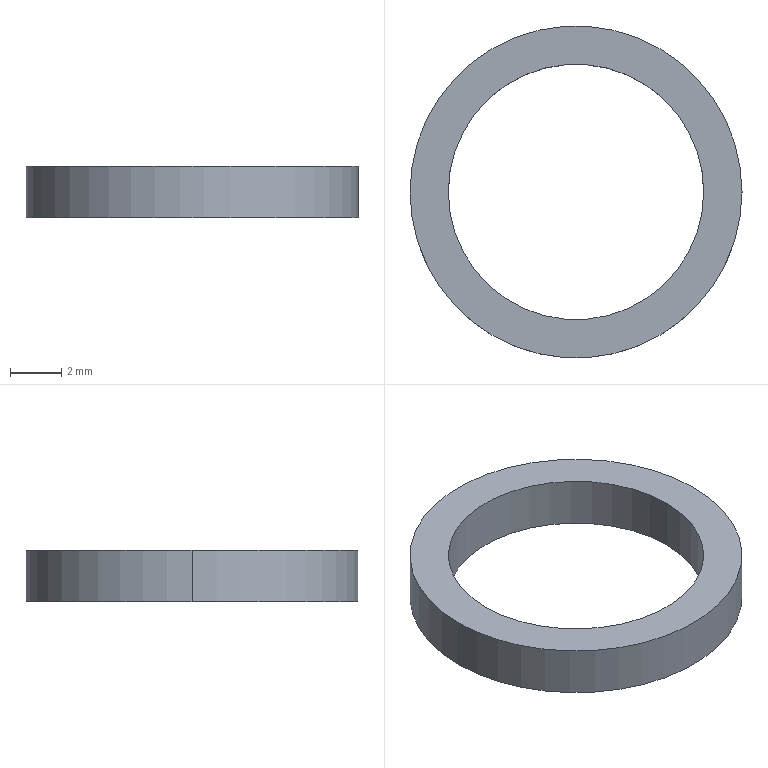Part | STEP file | 11-FG-B04311 | 1 solid | 6 faces | box 13 x 13 x 2 mm | volume 108.385 mm3 | cylinder 4 | plane 2 | commonest cylinder face diameters 10 x2 13 x2
STEP:
#1=CARTESIAN_POINT('',(-5.,0.,2.));
#2=VERTEX_POINT('',#1);
#3=CARTESIAN_POINT('',(5.,0.,2.));
#4=VERTEX_POINT('',#3);
#5=CARTESIAN_POINT('',(0.,0.,2.));
#6=DIRECTION('',(0.,0.,1.));
#7=DIRECTION('',(1.,0.,0.));
#8=AXIS2_PLACEMENT_3D('',#5,#6,#7);
#9=CIRCLE('',#8,5.);
#10=EDGE_CURVE('',#2,#4,#9,.T.);
#11=ORIENTED_EDGE('',*,*,#10,.T.);
#12=CARTESIAN_POINT('',(5.,0.,0.));
#13=VERTEX_POINT('',#12);
#14=CARTESIAN_POINT('',(5.,0.,2.));
#15=DIRECTION('',(0.,0.,-1.));
#16=VECTOR('',#15,1000.);
#17=LINE('',#14,#16);
#18=EDGE_CURVE('',#4,#13,#17,.T.);
#19=ORIENTED_EDGE('',*,*,#18,.T.);
#20=CARTESIAN_POINT('',(-5.,0.,0.));
#21=VERTEX_POINT('',#20);
#22=CARTESIAN_POINT('',(0.,0.,0.));
#23=DIRECTION('',(0.,0.,1.));
#24=DIRECTION('',(1.,0.,0.));
#25=AXIS2_PLACEMENT_3D('',#22,#23,#24);
#26=CIRCLE('',#25,5.);
#27=EDGE_CURVE('',#21,#13,#26,.T.);
#28=ORIENTED_EDGE('',*,*,#27,.F.);
#29=CARTESIAN_POINT('',(-5.,0.,2.));
#30=DIRECTION('',(0.,0.,-1.));
#31=VECTOR('',#30,1000.);
#32=LINE('',#29,#31);
#33=EDGE_CURVE('',#2,#21,#32,.T.);
#34=ORIENTED_EDGE('',*,*,#33,.F.);
#35=EDGE_LOOP('',(#11,#19,#28,#34));
#36=FACE_OUTER_BOUND('',#35,.T.);
#37=CARTESIAN_POINT('',(0.,0.,2.));
#38=DIRECTION('',(0.,0.,-1.));
#39=DIRECTION('',(-1.,0.,0.));
#40=AXIS2_PLACEMENT_3D('',#37,#38,#39);
#41=CYLINDRICAL_SURFACE('',#40,5.);
#42=ADVANCED_FACE('',(#36),#41,.F.);
#43=CARTESIAN_POINT('',(6.5,0.,2.));
#44=VERTEX_POINT('',#43);
#45=CARTESIAN_POINT('',(-6.5,0.,2.));
#46=VERTEX_POINT('',#45);
#47=CARTESIAN_POINT('',(0.,0.,2.));
#48=DIRECTION('',(0.,0.,1.));
#49=DIRECTION('',(1.,0.,0.));
#50=AXIS2_PLACEMENT_3D('',#47,#48,#49);
#51=CIRCLE('',#50,6.5);
#52=EDGE_CURVE('',#44,#46,#51,.T.);
#53=ORIENTED_EDGE('',*,*,#52,.F.);
#54=CARTESIAN_POINT('',(6.5,0.,0.));
#55=VERTEX_POINT('',#54);
#56=CARTESIAN_POINT('',(6.5,0.,2.));
#57=DIRECTION('',(0.,0.,-1.));
#58=VECTOR('',#57,1000.);
#59=LINE('',#56,#58);
#60=EDGE_CURVE('',#44,#55,#59,.T.);
#61=ORIENTED_EDGE('',*,*,#60,.T.);
#62=CARTESIAN_POINT('',(-6.5,0.,0.));
#63=VERTEX_POINT('',#62);
#64=CARTESIAN_POINT('',(0.,0.,0.));
#65=DIRECTION('',(0.,0.,1.));
#66=DIRECTION('',(1.,0.,0.));
#67=AXIS2_PLACEMENT_3D('',#64,#65,#66);
#68=CIRCLE('',#67,6.5);
#69=EDGE_CURVE('',#55,#63,#68,.T.);
#70=ORIENTED_EDGE('',*,*,#69,.T.);
#71=CARTESIAN_POINT('',(-6.5,0.,2.));
#72=DIRECTION('',(0.,0.,-1.));
#73=VECTOR('',#72,1000.);
#74=LINE('',#71,#73);
#75=EDGE_CURVE('',#46,#63,#74,.T.);
#76=ORIENTED_EDGE('',*,*,#75,.F.);
#77=EDGE_LOOP('',(#53,#61,#70,#76));
#78=FACE_OUTER_BOUND('',#77,.T.);
#79=CARTESIAN_POINT('',(0.,0.,2.));
#80=DIRECTION('',(0.,0.,-1.));
#81=DIRECTION('',(-1.,0.,0.));
#82=AXIS2_PLACEMENT_3D('',#79,#80,#81);
#83=CYLINDRICAL_SURFACE('',#82,6.5);
#84=ADVANCED_FACE('',(#78),#83,.T.);
#85=CARTESIAN_POINT('',(0.,0.,2.));
#86=DIRECTION('',(0.,0.,1.));
#87=DIRECTION('',(1.,0.,0.));
#88=AXIS2_PLACEMENT_3D('',#85,#86,#87);
#89=CIRCLE('',#88,6.5);
#90=EDGE_CURVE('',#46,#44,#89,.T.);
#91=ORIENTED_EDGE('',*,*,#90,.T.);
#92=ORIENTED_EDGE('',*,*,#52,.T.);
#93=EDGE_LOOP('',(#91,#92));
#94=FACE_OUTER_BOUND('',#93,.T.);
#95=ORIENTED_EDGE('',*,*,#10,.F.);
#96=CARTESIAN_POINT('',(0.,0.,2.));
#97=DIRECTION('',(0.,0.,1.));
#98=DIRECTION('',(1.,0.,0.));
#99=AXIS2_PLACEMENT_3D('',#96,#97,#98);
#100=CIRCLE('',#99,5.);
#101=EDGE_CURVE('',#4,#2,#100,.T.);
#102=ORIENTED_EDGE('',*,*,#101,.F.);
#103=EDGE_LOOP('',(#95,#102));
#104=FACE_BOUND('',#103,.T.);
#105=CARTESIAN_POINT('',(0.,0.,2.));
#106=DIRECTION('',(0.,0.,1.));
#107=DIRECTION('',(1.,0.,0.));
#108=AXIS2_PLACEMENT_3D('',#105,#106,#107);
#109=PLANE('',#108);
#110=ADVANCED_FACE('',(#94,#104),#109,.T.);
#111=CARTESIAN_POINT('',(0.,0.,0.));
#112=DIRECTION('',(0.,0.,1.));
#113=DIRECTION('',(1.,0.,0.));
#114=AXIS2_PLACEMENT_3D('',#111,#112,#113);
#115=CIRCLE('',#114,6.5);
#116=EDGE_CURVE('',#63,#55,#115,.T.);
#117=ORIENTED_EDGE('',*,*,#116,.F.);
#118=ORIENTED_EDGE('',*,*,#69,.F.);
#119=EDGE_LOOP('',(#117,#118));
#120=FACE_OUTER_BOUND('',#119,.T.);
#121=ORIENTED_EDGE('',*,*,#27,.T.);
#122=CARTESIAN_POINT('',(0.,0.,0.));
#123=DIRECTION('',(0.,0.,1.));
#124=DIRECTION('',(1.,0.,0.));
#125=AXIS2_PLACEMENT_3D('',#122,#123,#124);
#126=CIRCLE('',#125,5.);
#127=EDGE_CURVE('',#13,#21,#126,.T.);
#128=ORIENTED_EDGE('',*,*,#127,.T.);
#129=EDGE_LOOP('',(#121,#128));
#130=FACE_BOUND('',#129,.T.);
#131=CARTESIAN_POINT('',(0.,0.,0.));
#132=DIRECTION('',(0.,0.,1.));
#133=DIRECTION('',(1.,0.,0.));
#134=AXIS2_PLACEMENT_3D('',#131,#132,#133);
#135=PLANE('',#134);
#136=ADVANCED_FACE('',(#120,#130),#135,.F.);
#137=ORIENTED_EDGE('',*,*,#60,.F.);
#138=ORIENTED_EDGE('',*,*,#90,.F.);
#139=ORIENTED_EDGE('',*,*,#75,.T.);
#140=ORIENTED_EDGE('',*,*,#116,.T.);
#141=EDGE_LOOP('',(#137,#138,#139,#140));
#142=FACE_OUTER_BOUND('',#141,.T.);
#143=CARTESIAN_POINT('',(0.,0.,2.));
#144=DIRECTION('',(0.,0.,-1.));
#145=DIRECTION('',(-1.,0.,0.));
#146=AXIS2_PLACEMENT_3D('',#143,#144,#145);
#147=CYLINDRICAL_SURFACE('',#146,6.5);
#148=ADVANCED_FACE('',(#142),#147,.T.);
#149=ORIENTED_EDGE('',*,*,#18,.F.);
#150=ORIENTED_EDGE('',*,*,#101,.T.);
#151=ORIENTED_EDGE('',*,*,#33,.T.);
#152=ORIENTED_EDGE('',*,*,#127,.F.);
#153=EDGE_LOOP('',(#149,#150,#151,#152));
#154=FACE_OUTER_BOUND('',#153,.T.);
#155=CARTESIAN_POINT('',(0.,0.,2.));
#156=DIRECTION('',(0.,0.,-1.));
#157=DIRECTION('',(-1.,0.,0.));
#158=AXIS2_PLACEMENT_3D('',#155,#156,#157);
#159=CYLINDRICAL_SURFACE('',#158,5.);
#160=ADVANCED_FACE('',(#154),#159,.F.);
#161=CLOSED_SHELL('',(#42,#84,#110,#136,#148,#160));
#162=MANIFOLD_SOLID_BREP('',#161);
#163=CARTESIAN_POINT('',(0.,0.,0.));
#164=DIRECTION('',(0.,0.,1.));
#165=DIRECTION('',(1.,0.,0.));
#166=AXIS2_PLACEMENT_3D('',#163,#164,#165);
#167=(LENGTH_UNIT()NAMED_UNIT(*)SI_UNIT(.MILLI.,.METRE.));
#168=UNCERTAINTY_MEASURE_WITH_UNIT(LENGTH_MEASURE(0.00001),#167,'','');
#169=(NAMED_UNIT(*)PLANE_ANGLE_UNIT()SI_UNIT($,.RADIAN.));
#170=(NAMED_UNIT(*)SI_UNIT($,.STERADIAN.)SOLID_ANGLE_UNIT());
#171=(GEOMETRIC_REPRESENTATION_CONTEXT(3)GLOBAL_UNCERTAINTY_ASSIGNED_CONTEXT((#168))GLOBAL_UNIT_ASSIGNED_CONTEXT((#167,#169,#170))REPRESENTATION_CONTEXT('',''));
#172=ADVANCED_BREP_SHAPE_REPRESENTATION('',(#162,#166),#171);